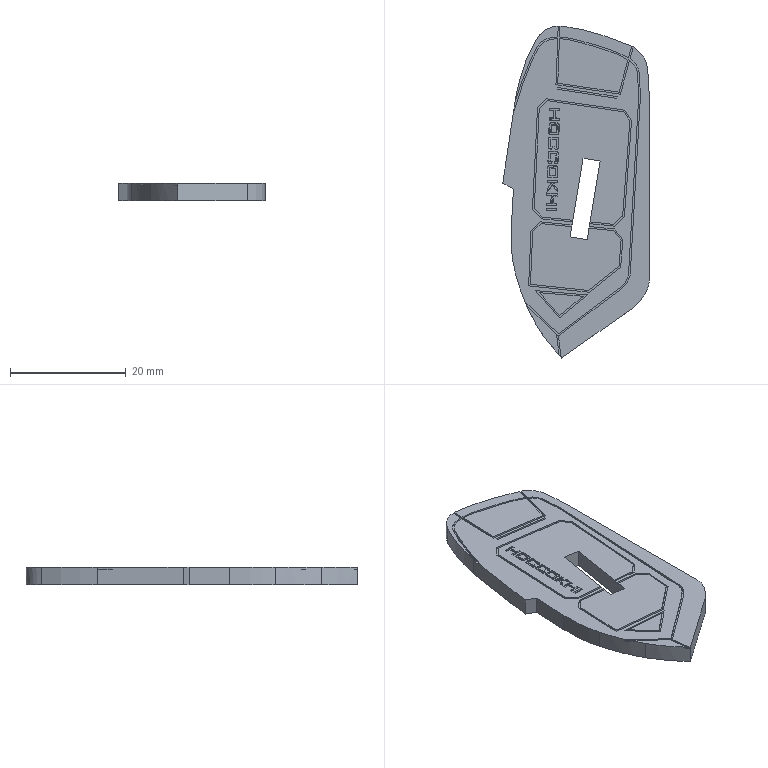Part | SolidWorks | features BaseBody 1 | 1 solid | 215 faces | box 25.301 x 57.359 x 3 mm | volume 3340 mm3 | plane 170 | spline 45